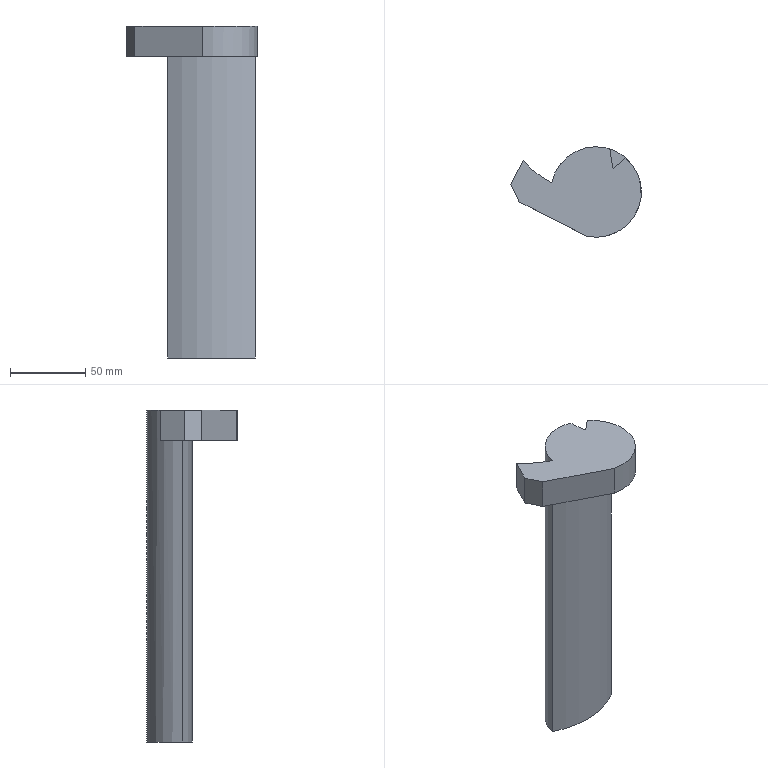Part | SolidWorks | features BaseBody 1 | 1 solid | 13 faces | box 86.498 x 60 x 220 mm | volume 320268 mm3 | plane 8 | cylinder 5 | commonest cylinder face diameters 120 x4 60 x1
STEP:
#1=CARTESIAN_POINT('',(238.508,899.452,-684.893));
#2=VERTEX_POINT('',#1);
#3=CARTESIAN_POINT('',(219.563,914.153,-684.893));
#4=VERTEX_POINT('',#3);
#5=CARTESIAN_POINT('',(265.077,953.249,-684.893));
#6=DIRECTION('',(0.,0.,-1.));
#7=DIRECTION('',(1.,0.,0.));
#8=AXIS2_PLACEMENT_3D('',#5,#6,#7);
#9=CIRCLE('',#8,60.);
#10=EDGE_CURVE('',#2,#4,#9,.T.);
#11=ORIENTED_EDGE('',*,*,#10,.T.);
#12=CARTESIAN_POINT('',(219.563,914.153,-664.893));
#13=VERTEX_POINT('',#12);
#14=CARTESIAN_POINT('',(219.563,914.153,-634.893));
#15=DIRECTION('',(0.,0.,-1.));
#16=VECTOR('',#15,1000.);
#17=LINE('',#14,#16);
#18=EDGE_CURVE('',#13,#4,#17,.T.);
#19=ORIENTED_EDGE('',*,*,#18,.F.);
#20=CARTESIAN_POINT('',(238.508,899.452,-664.893));
#21=VERTEX_POINT('',#20);
#22=CARTESIAN_POINT('',(265.077,953.249,-664.893));
#23=DIRECTION('',(0.,0.,-1.));
#24=DIRECTION('',(1.,0.,0.));
#25=AXIS2_PLACEMENT_3D('',#22,#23,#24);
#26=CIRCLE('',#25,60.);
#27=EDGE_CURVE('',#21,#13,#26,.T.);
#28=ORIENTED_EDGE('',*,*,#27,.F.);
#29=CARTESIAN_POINT('',(238.508,899.452,-759.893));
#30=DIRECTION('',(0.,0.,1.));
#31=VECTOR('',#30,1000.);
#32=LINE('',#29,#31);
#33=EDGE_CURVE('',#2,#21,#32,.T.);
#34=ORIENTED_EDGE('',*,*,#33,.F.);
#35=EDGE_LOOP('',(#11,#19,#28,#34));
#36=FACE_OUTER_BOUND('',#35,.T.);
#37=CARTESIAN_POINT('',(265.077,953.249,-934.893));
#38=DIRECTION('',(0.,0.,1.));
#39=DIRECTION('',(-0.9989,-0.04661,0.));
#40=AXIS2_PLACEMENT_3D('',#37,#38,#39);
#41=CYLINDRICAL_SURFACE('',#40,60.);
#42=ADVANCED_FACE('',(#36),#41,.F.);
#43=CARTESIAN_POINT('',(277.484,921.026,-684.893));
#44=VERTEX_POINT('',#43);
#45=CARTESIAN_POINT('',(274.431,922.589,-684.893));
#46=VERTEX_POINT('',#45);
#47=CARTESIAN_POINT('',(277.484,921.026,-684.893));
#48=DIRECTION('',(-0.8902,0.4556,0.));
#49=VECTOR('',#48,1000.);
#50=LINE('',#47,#49);
#51=EDGE_CURVE('',#44,#46,#50,.T.);
#52=ORIENTED_EDGE('',*,*,#51,.F.);
#53=CARTESIAN_POINT('',(279.192,908.736,-684.893));
#54=VERTEX_POINT('',#53);
#55=CARTESIAN_POINT('',(337.449,923.095,-684.893));
#56=DIRECTION('',(0.,0.,-1.));
#57=DIRECTION('',(-0.4556,-0.8902,0.));
#58=AXIS2_PLACEMENT_3D('',#55,#56,#57);
#59=CIRCLE('',#58,60.);
#60=EDGE_CURVE('',#54,#44,#59,.T.);
#61=ORIENTED_EDGE('',*,*,#60,.F.);
#62=CARTESIAN_POINT('',(287.784,915.755,-684.893));
#63=VERTEX_POINT('',#62);
#64=CARTESIAN_POINT('',(321.285,865.978,-684.893));
#65=DIRECTION('',(0.,0.,-1.));
#66=DIRECTION('',(1.,0.,0.));
#67=AXIS2_PLACEMENT_3D('',#64,#65,#66);
#68=CIRCLE('',#67,60.);
#69=EDGE_CURVE('',#54,#63,#68,.T.);
#70=ORIENTED_EDGE('',*,*,#69,.T.);
#71=CARTESIAN_POINT('',(267.874,893.314,-684.893));
#72=DIRECTION('',(0.,0.,-1.));
#73=DIRECTION('',(-0.9989,-0.04661,0.));
#74=AXIS2_PLACEMENT_3D('',#71,#72,#73);
#75=CIRCLE('',#74,30.);
#76=EDGE_CURVE('',#46,#63,#75,.T.);
#77=ORIENTED_EDGE('',*,*,#76,.F.);
#78=EDGE_LOOP('',(#52,#61,#70,#77));
#79=FACE_OUTER_BOUND('',#78,.T.);
#80=CARTESIAN_POINT('',(267.874,893.314,-684.893));
#81=DIRECTION('',(0.,0.,-1.));
#82=DIRECTION('',(0.,-1.,0.));
#83=AXIS2_PLACEMENT_3D('',#80,#81,#82);
#84=PLANE('',#83);
#85=ADVANCED_FACE('',(#79),#84,.F.);
#86=CARTESIAN_POINT('',(238.508,899.452,-884.893));
#87=VERTEX_POINT('',#86);
#88=CARTESIAN_POINT('',(296.54,902.16,-884.893));
#89=VERTEX_POINT('',#88);
#90=CARTESIAN_POINT('',(267.874,893.314,-884.893));
#91=DIRECTION('',(0.,0.,-1.));
#92=DIRECTION('',(-0.9989,-0.04661,0.));
#93=AXIS2_PLACEMENT_3D('',#90,#91,#92);
#94=CIRCLE('',#93,30.);
#95=EDGE_CURVE('',#87,#89,#94,.T.);
#96=ORIENTED_EDGE('',*,*,#95,.T.);
#97=CARTESIAN_POINT('',(265.077,953.249,-884.893));
#98=DIRECTION('',(0.,0.,-1.));
#99=DIRECTION('',(-0.9989,-0.04661,0.));
#100=AXIS2_PLACEMENT_3D('',#97,#98,#99);
#101=CIRCLE('',#100,60.);
#102=EDGE_CURVE('',#89,#87,#101,.T.);
#103=ORIENTED_EDGE('',*,*,#102,.T.);
#104=EDGE_LOOP('',(#96,#103));
#105=FACE_OUTER_BOUND('',#104,.T.);
#106=CARTESIAN_POINT('',(267.874,893.314,-884.893));
#107=DIRECTION('',(0.,0.,-1.));
#108=DIRECTION('',(0.,-1.,0.));
#109=AXIS2_PLACEMENT_3D('',#106,#107,#108);
#110=PLANE('',#109);
#111=ADVANCED_FACE('',(#105),#110,.T.);
#112=CARTESIAN_POINT('',(296.54,902.16,-684.893));
#113=VERTEX_POINT('',#112);
#114=CARTESIAN_POINT('',(265.077,953.249,-684.893));
#115=DIRECTION('',(0.,0.,-1.));
#116=DIRECTION('',(-0.9989,-0.04661,0.));
#117=AXIS2_PLACEMENT_3D('',#114,#115,#116);
#118=CIRCLE('',#117,60.);
#119=EDGE_CURVE('',#113,#2,#118,.T.);
#120=ORIENTED_EDGE('',*,*,#119,.T.);
#121=CARTESIAN_POINT('',(238.508,899.452,-884.893));
#122=DIRECTION('',(0.,0.,1.));
#123=VECTOR('',#122,1000.);
#124=LINE('',#121,#123);
#125=EDGE_CURVE('',#87,#2,#124,.T.);
#126=ORIENTED_EDGE('',*,*,#125,.F.);
#127=ORIENTED_EDGE('',*,*,#102,.F.);
#128=CARTESIAN_POINT('',(296.54,902.16,-884.893));
#129=DIRECTION('',(0.,0.,1.));
#130=VECTOR('',#129,1000.);
#131=LINE('',#128,#130);
#132=EDGE_CURVE('',#89,#113,#131,.T.);
#133=ORIENTED_EDGE('',*,*,#132,.T.);
#134=EDGE_LOOP('',(#120,#126,#127,#133));
#135=FACE_OUTER_BOUND('',#134,.T.);
#136=CARTESIAN_POINT('',(265.077,953.249,-884.893));
#137=DIRECTION('',(0.,0.,1.));
#138=DIRECTION('',(1.,0.,0.));
#139=AXIS2_PLACEMENT_3D('',#136,#137,#138);
#140=CYLINDRICAL_SURFACE('',#139,60.);
#141=ADVANCED_FACE('',(#135),#140,.T.);
#142=CARTESIAN_POINT('',(211.376,898.158,-664.893));
#143=VERTEX_POINT('',#142);
#144=CARTESIAN_POINT('',(234.373,943.09,-664.893));
#145=DIRECTION('',(-0.4556,-0.8902,0.));
#146=VECTOR('',#145,1000.);
#147=LINE('',#144,#146);
#148=EDGE_CURVE('',#13,#143,#147,.T.);
#149=ORIENTED_EDGE('',*,*,#148,.T.);
#150=CARTESIAN_POINT('',(216.807,886.819,-664.893));
#151=VERTEX_POINT('',#150);
#152=CARTESIAN_POINT('',(189.653,943.511,-664.893));
#153=DIRECTION('',(0.432,-0.9019,0.));
#154=VECTOR('',#153,1000.);
#155=LINE('',#152,#154);
#156=EDGE_CURVE('',#143,#151,#155,.T.);
#157=ORIENTED_EDGE('',*,*,#156,.T.);
#158=CARTESIAN_POINT('',(261.316,864.04,-664.893));
#159=VERTEX_POINT('',#158);
#160=CARTESIAN_POINT('',(261.316,864.04,-664.893));
#161=DIRECTION('',(0.8902,-0.4556,0.));
#162=VECTOR('',#161,1000.);
#163=LINE('',#160,#162);
#164=EDGE_CURVE('',#151,#159,#163,.T.);
#165=ORIENTED_EDGE('',*,*,#164,.T.);
#166=CARTESIAN_POINT('',(287.784,915.755,-664.893));
#167=VERTEX_POINT('',#166);
#168=CARTESIAN_POINT('',(267.874,893.314,-664.893));
#169=DIRECTION('',(0.,0.,1.));
#170=DIRECTION('',(1.,0.,0.));
#171=AXIS2_PLACEMENT_3D('',#168,#169,#170);
#172=CIRCLE('',#171,30.);
#173=EDGE_CURVE('',#159,#167,#172,.T.);
#174=ORIENTED_EDGE('',*,*,#173,.T.);
#175=CARTESIAN_POINT('',(279.192,908.736,-664.893));
#176=VERTEX_POINT('',#175);
#177=CARTESIAN_POINT('',(321.285,865.978,-664.893));
#178=DIRECTION('',(0.,0.,1.));
#179=DIRECTION('',(1.,0.,0.));
#180=AXIS2_PLACEMENT_3D('',#177,#178,#179);
#181=CIRCLE('',#180,60.);
#182=EDGE_CURVE('',#167,#176,#181,.T.);
#183=ORIENTED_EDGE('',*,*,#182,.T.);
#184=CARTESIAN_POINT('',(277.484,921.026,-664.893));
#185=VERTEX_POINT('',#184);
#186=CARTESIAN_POINT('',(337.449,923.095,-664.893));
#187=DIRECTION('',(0.,0.,-1.));
#188=DIRECTION('',(1.,0.,0.));
#189=AXIS2_PLACEMENT_3D('',#186,#187,#188);
#190=CIRCLE('',#189,60.);
#191=EDGE_CURVE('',#176,#185,#190,.T.);
#192=ORIENTED_EDGE('',*,*,#191,.T.);
#193=CARTESIAN_POINT('',(274.431,922.589,-664.893));
#194=VERTEX_POINT('',#193);
#195=CARTESIAN_POINT('',(277.484,921.026,-664.893));
#196=DIRECTION('',(-0.8902,0.4556,0.));
#197=VECTOR('',#196,1000.);
#198=LINE('',#195,#197);
#199=EDGE_CURVE('',#185,#194,#198,.T.);
#200=ORIENTED_EDGE('',*,*,#199,.T.);
#201=CARTESIAN_POINT('',(267.874,893.314,-664.893));
#202=DIRECTION('',(0.,0.,-1.));
#203=DIRECTION('',(1.,0.,0.));
#204=AXIS2_PLACEMENT_3D('',#201,#202,#203);
#205=CIRCLE('',#204,30.);
#206=EDGE_CURVE('',#21,#194,#205,.T.);
#207=ORIENTED_EDGE('',*,*,#206,.F.);
#208=ORIENTED_EDGE('',*,*,#27,.T.);
#209=EDGE_LOOP('',(#149,#157,#165,#174,#183,#192,#200,#207,#208));
#210=FACE_OUTER_BOUND('',#209,.T.);
#211=CARTESIAN_POINT('',(267.874,893.314,-664.893));
#212=DIRECTION('',(0.,0.,1.));
#213=DIRECTION('',(1.,0.,0.));
#214=AXIS2_PLACEMENT_3D('',#211,#212,#213);
#215=PLANE('',#214);
#216=ADVANCED_FACE('',(#210),#215,.T.);
#217=ORIENTED_EDGE('',*,*,#148,.F.);
#218=ORIENTED_EDGE('',*,*,#18,.T.);
#219=CARTESIAN_POINT('',(211.376,898.158,-684.893));
#220=VERTEX_POINT('',#219);
#221=CARTESIAN_POINT('',(221.139,917.233,-684.893));
#222=DIRECTION('',(-0.4556,-0.8902,0.));
#223=VECTOR('',#222,1000.);
#224=LINE('',#221,#223);
#225=EDGE_CURVE('',#4,#220,#224,.T.);
#226=ORIENTED_EDGE('',*,*,#225,.T.);
#227=CARTESIAN_POINT('',(211.376,898.158,-634.893));
#228=DIRECTION('',(0.,0.,-1.));
#229=VECTOR('',#228,1000.);
#230=LINE('',#227,#229);
#231=EDGE_CURVE('',#143,#220,#230,.T.);
#232=ORIENTED_EDGE('',*,*,#231,.F.);
#233=EDGE_LOOP('',(#217,#218,#226,#232));
#234=FACE_OUTER_BOUND('',#233,.T.);
#235=CARTESIAN_POINT('',(234.373,943.09,-634.893));
#236=DIRECTION('',(0.8902,-0.4556,0.));
#237=DIRECTION('',(0.,0.,-1.));
#238=AXIS2_PLACEMENT_3D('',#235,#236,#237);
#239=PLANE('',#238);
#240=ADVANCED_FACE('',(#234),#239,.F.);
#241=ORIENTED_EDGE('',*,*,#60,.T.);
#242=CARTESIAN_POINT('',(277.484,921.026,-634.893));
#243=DIRECTION('',(0.,0.,-1.));
#244=VECTOR('',#243,1000.);
#245=LINE('',#242,#244);
#246=EDGE_CURVE('',#185,#44,#245,.T.);
#247=ORIENTED_EDGE('',*,*,#246,.F.);
#248=ORIENTED_EDGE('',*,*,#191,.F.);
#249=CARTESIAN_POINT('',(279.192,908.736,-634.893));
#250=DIRECTION('',(0.,0.,-1.));
#251=VECTOR('',#250,1000.);
#252=LINE('',#249,#251);
#253=EDGE_CURVE('',#176,#54,#252,.T.);
#254=ORIENTED_EDGE('',*,*,#253,.T.);
#255=EDGE_LOOP('',(#241,#247,#248,#254));
#256=FACE_OUTER_BOUND('',#255,.T.);
#257=CARTESIAN_POINT('',(337.449,923.095,-634.893));
#258=DIRECTION('',(0.,0.,-1.));
#259=DIRECTION('',(0.4556,0.8902,0.));
#260=AXIS2_PLACEMENT_3D('',#257,#258,#259);
#261=CYLINDRICAL_SURFACE('',#260,60.);
#262=ADVANCED_FACE('',(#256),#261,.F.);
#263=CARTESIAN_POINT('',(216.807,886.819,-684.893));
#264=VERTEX_POINT('',#263);
#265=CARTESIAN_POINT('',(261.316,864.04,-684.893));
#266=VERTEX_POINT('',#265);
#267=CARTESIAN_POINT('',(261.316,864.04,-684.893));
#268=DIRECTION('',(0.8902,-0.4556,0.));
#269=VECTOR('',#268,1000.);
#270=LINE('',#267,#269);
#271=EDGE_CURVE('',#264,#266,#270,.T.);
#272=ORIENTED_EDGE('',*,*,#271,.T.);
#273=CARTESIAN_POINT('',(261.316,864.04,-634.893));
#274=DIRECTION('',(0.,0.,-1.));
#275=VECTOR('',#274,1000.);
#276=LINE('',#273,#275);
#277=EDGE_CURVE('',#159,#266,#276,.T.);
#278=ORIENTED_EDGE('',*,*,#277,.F.);
#279=ORIENTED_EDGE('',*,*,#164,.F.);
#280=CARTESIAN_POINT('',(216.807,886.819,-634.893));
#281=DIRECTION('',(0.,0.,-1.));
#282=VECTOR('',#281,1000.);
#283=LINE('',#280,#282);
#284=EDGE_CURVE('',#151,#264,#283,.T.);
#285=ORIENTED_EDGE('',*,*,#284,.T.);
#286=EDGE_LOOP('',(#272,#278,#279,#285));
#287=FACE_OUTER_BOUND('',#286,.T.);
#288=CARTESIAN_POINT('',(261.316,864.04,-634.893));
#289=DIRECTION('',(0.4556,0.8902,0.));
#290=DIRECTION('',(0.,0.,-1.));
#291=AXIS2_PLACEMENT_3D('',#288,#289,#290);
#292=PLANE('',#291);
#293=ADVANCED_FACE('',(#287),#292,.F.);
#294=CARTESIAN_POINT('',(189.653,943.511,-684.893));
#295=DIRECTION('',(0.432,-0.9019,0.));
#296=VECTOR('',#295,1000.);
#297=LINE('',#294,#296);
#298=EDGE_CURVE('',#220,#264,#297,.T.);
#299=ORIENTED_EDGE('',*,*,#298,.T.);
#300=ORIENTED_EDGE('',*,*,#284,.F.);
#301=ORIENTED_EDGE('',*,*,#156,.F.);
#302=ORIENTED_EDGE('',*,*,#231,.T.);
#303=EDGE_LOOP('',(#299,#300,#301,#302));
#304=FACE_OUTER_BOUND('',#303,.T.);
#305=CARTESIAN_POINT('',(189.653,943.511,-634.893));
#306=DIRECTION('',(0.9019,0.432,0.));
#307=DIRECTION('',(0.,0.,-1.));
#308=AXIS2_PLACEMENT_3D('',#305,#306,#307);
#309=PLANE('',#308);
#310=ADVANCED_FACE('',(#304),#309,.F.);
#311=ORIENTED_EDGE('',*,*,#10,.F.);
#312=ORIENTED_EDGE('',*,*,#119,.F.);
#313=CARTESIAN_POINT('',(267.874,893.314,-684.893));
#314=DIRECTION('',(0.,0.,-1.));
#315=DIRECTION('',(1.,0.,0.));
#316=AXIS2_PLACEMENT_3D('',#313,#314,#315);
#317=CIRCLE('',#316,30.);
#318=EDGE_CURVE('',#113,#266,#317,.T.);
#319=ORIENTED_EDGE('',*,*,#318,.T.);
#320=ORIENTED_EDGE('',*,*,#271,.F.);
#321=ORIENTED_EDGE('',*,*,#298,.F.);
#322=ORIENTED_EDGE('',*,*,#225,.F.);
#323=EDGE_LOOP('',(#311,#312,#319,#320,#321,#322));
#324=FACE_OUTER_BOUND('',#323,.T.);
#325=CARTESIAN_POINT('',(267.874,893.314,-684.893));
#326=DIRECTION('',(0.,0.,1.));
#327=DIRECTION('',(1.,0.,0.));
#328=AXIS2_PLACEMENT_3D('',#325,#326,#327);
#329=PLANE('',#328);
#330=ADVANCED_FACE('',(#324),#329,.F.);
#331=ORIENTED_EDGE('',*,*,#69,.F.);
#332=ORIENTED_EDGE('',*,*,#253,.F.);
#333=ORIENTED_EDGE('',*,*,#182,.F.);
#334=CARTESIAN_POINT('',(287.784,915.755,-884.893));
#335=DIRECTION('',(0.,0.,-1.));
#336=VECTOR('',#335,1000.);
#337=LINE('',#334,#336);
#338=EDGE_CURVE('',#167,#63,#337,.T.);
#339=ORIENTED_EDGE('',*,*,#338,.T.);
#340=EDGE_LOOP('',(#331,#332,#333,#339));
#341=FACE_OUTER_BOUND('',#340,.T.);
#342=CARTESIAN_POINT('',(321.285,865.978,-884.893));
#343=DIRECTION('',(0.,0.,1.));
#344=DIRECTION('',(-0.4556,-0.8902,0.));
#345=AXIS2_PLACEMENT_3D('',#342,#343,#344);
#346=CYLINDRICAL_SURFACE('',#345,60.);
#347=ADVANCED_FACE('',(#341),#346,.T.);
#348=ORIENTED_EDGE('',*,*,#318,.F.);
#349=ORIENTED_EDGE('',*,*,#132,.F.);
#350=ORIENTED_EDGE('',*,*,#95,.F.);
#351=ORIENTED_EDGE('',*,*,#125,.T.);
#352=ORIENTED_EDGE('',*,*,#33,.T.);
#353=ORIENTED_EDGE('',*,*,#206,.T.);
#354=CARTESIAN_POINT('',(274.431,922.589,-634.893));
#355=DIRECTION('',(0.,0.,-1.));
#356=VECTOR('',#355,1000.);
#357=LINE('',#354,#356);
#358=EDGE_CURVE('',#194,#46,#357,.T.);
#359=ORIENTED_EDGE('',*,*,#358,.T.);
#360=ORIENTED_EDGE('',*,*,#76,.T.);
#361=ORIENTED_EDGE('',*,*,#338,.F.);
#362=ORIENTED_EDGE('',*,*,#173,.F.);
#363=ORIENTED_EDGE('',*,*,#277,.T.);
#364=EDGE_LOOP('',(#348,#349,#350,#351,#352,#353,#359,#360,#361,#362,#363));
#365=FACE_OUTER_BOUND('',#364,.T.);
#366=CARTESIAN_POINT('',(267.874,893.314,-884.893));
#367=DIRECTION('',(0.,0.,1.));
#368=DIRECTION('',(-0.4556,-0.8902,0.));
#369=AXIS2_PLACEMENT_3D('',#366,#367,#368);
#370=CYLINDRICAL_SURFACE('',#369,30.);
#371=ADVANCED_FACE('',(#365),#370,.T.);
#372=ORIENTED_EDGE('',*,*,#358,.F.);
#373=ORIENTED_EDGE('',*,*,#199,.F.);
#374=ORIENTED_EDGE('',*,*,#246,.T.);
#375=ORIENTED_EDGE('',*,*,#51,.T.);
#376=EDGE_LOOP('',(#372,#373,#374,#375));
#377=FACE_OUTER_BOUND('',#376,.T.);
#378=CARTESIAN_POINT('',(277.484,921.026,-634.893));
#379=DIRECTION('',(-0.4556,-0.8902,0.));
#380=DIRECTION('',(-0.8902,0.4556,0.));
#381=AXIS2_PLACEMENT_3D('',#378,#379,#380);
#382=PLANE('',#381);
#383=ADVANCED_FACE('',(#377),#382,.F.);
#384=CLOSED_SHELL('',(#42,#85,#111,#141,#216,#240,#262,#293,#310,#330,#347,#371,#383));
#385=MANIFOLD_SOLID_BREP('',#384);
#386=CARTESIAN_POINT('',(0.,0.,0.));
#387=DIRECTION('',(0.,0.,1.));
#388=DIRECTION('',(1.,0.,0.));
#389=AXIS2_PLACEMENT_3D('',#386,#387,#388);
#390=(LENGTH_UNIT()NAMED_UNIT(*)SI_UNIT(.MILLI.,.METRE.));
#391=UNCERTAINTY_MEASURE_WITH_UNIT(LENGTH_MEASURE(0.00001),#390,'','');
#392=(NAMED_UNIT(*)PLANE_ANGLE_UNIT()SI_UNIT($,.RADIAN.));
#393=(NAMED_UNIT(*)SI_UNIT($,.STERADIAN.)SOLID_ANGLE_UNIT());
#394=(GEOMETRIC_REPRESENTATION_CONTEXT(3)GLOBAL_UNCERTAINTY_ASSIGNED_CONTEXT((#391))GLOBAL_UNIT_ASSIGNED_CONTEXT((#390,#392,#393))REPRESENTATION_CONTEXT('',''));
#395=ADVANCED_BREP_SHAPE_REPRESENTATION('',(#385,#389),#394);